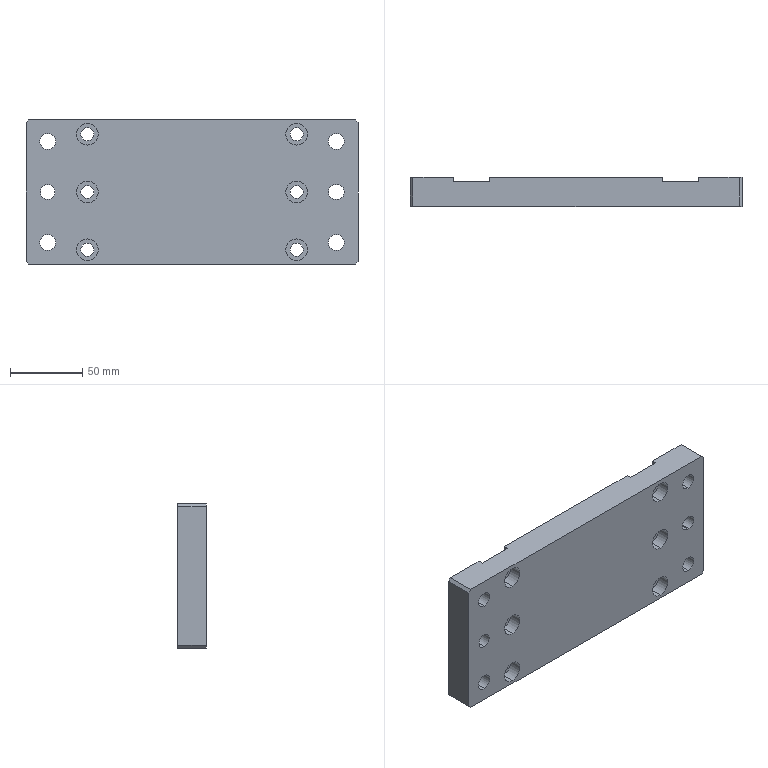Part | SolidWorks | features HoleWzd 4, Chamfer 1, Extrusion 1, ICE 1 | 1 solid | 74 faces | box 230 x 20 x 100 mm | volume 414284 mm3 | cylinder 44 | plane 30 | commonest cylinder face diameters 9 x12 15 x12 11 x8 18 x8 10 x4